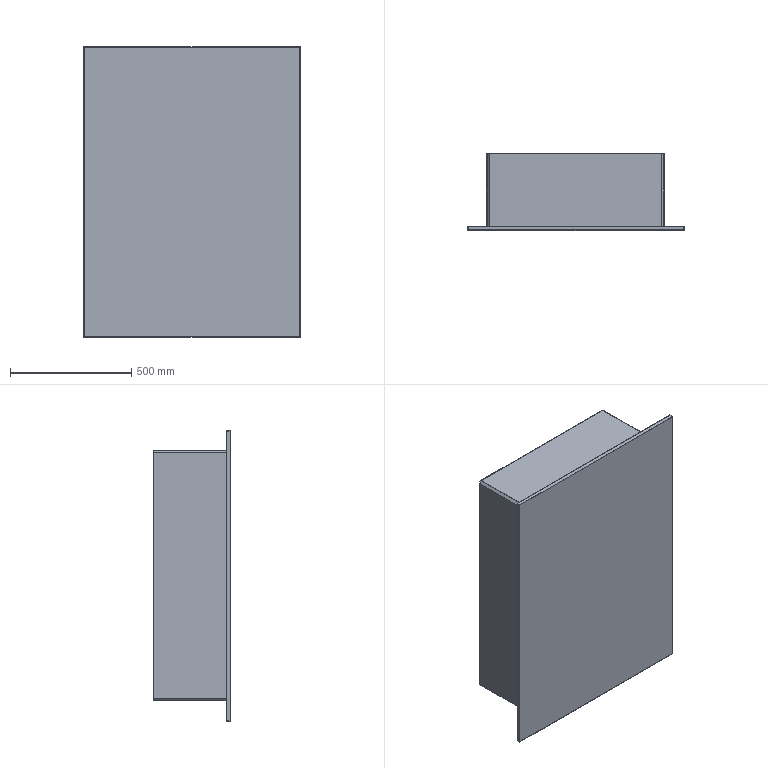Part | SolidWorks | features ICE 2, Chamfer 1, Extrusion 1, Shell 1 | 1 solid | 34 faces | box 892 x 317 x 1197 mm | volume 3890024 mm3 | plane 30 | cylinder 4 | commonest cylinder face diameters 59 x4
STEP:
#1=CARTESIAN_POINT('',(198.5,315.8,390.));
#2=VERTEX_POINT('',#1);
#3=CARTESIAN_POINT('',(198.5,315.8,449.));
#4=VERTEX_POINT('',#3);
#5=CARTESIAN_POINT('',(198.5,315.8,419.5));
#6=DIRECTION('',(0.,1.,0.));
#7=DIRECTION('',(0.,0.,1.));
#8=AXIS2_PLACEMENT_3D('',#5,#6,#7);
#9=CIRCLE('',#8,29.5);
#10=EDGE_CURVE('',#2,#4,#9,.T.);
#11=ORIENTED_EDGE('',*,*,#10,.F.);
#12=CARTESIAN_POINT('',(198.5,317.,390.));
#13=VERTEX_POINT('',#12);
#14=CARTESIAN_POINT('',(198.5,307.,390.));
#15=DIRECTION('',(0.,1.,0.));
#16=VECTOR('',#15,1000.);
#17=LINE('',#14,#16);
#18=EDGE_CURVE('',#2,#13,#17,.T.);
#19=ORIENTED_EDGE('',*,*,#18,.T.);
#20=CARTESIAN_POINT('',(198.5,317.,449.));
#21=VERTEX_POINT('',#20);
#22=CARTESIAN_POINT('',(198.5,317.,419.5));
#23=DIRECTION('',(0.,1.,0.));
#24=DIRECTION('',(0.,0.,1.));
#25=AXIS2_PLACEMENT_3D('',#22,#23,#24);
#26=CIRCLE('',#25,29.5);
#27=EDGE_CURVE('',#13,#21,#26,.T.);
#28=ORIENTED_EDGE('',*,*,#27,.T.);
#29=CARTESIAN_POINT('',(198.5,307.,449.));
#30=DIRECTION('',(0.,1.,0.));
#31=VECTOR('',#30,1000.);
#32=LINE('',#29,#31);
#33=EDGE_CURVE('',#4,#21,#32,.T.);
#34=ORIENTED_EDGE('',*,*,#33,.F.);
#35=EDGE_LOOP('',(#11,#19,#28,#34));
#36=FACE_OUTER_BOUND('',#35,.T.);
#37=CARTESIAN_POINT('',(198.5,307.,419.5));
#38=DIRECTION('',(0.,1.,0.));
#39=DIRECTION('',(0.,0.,1.));
#40=AXIS2_PLACEMENT_3D('',#37,#38,#39);
#41=CYLINDRICAL_SURFACE('',#40,29.5);
#42=ADVANCED_FACE('',(#36),#41,.F.);
#43=CARTESIAN_POINT('',(-201.5,315.8,390.));
#44=VERTEX_POINT('',#43);
#45=CARTESIAN_POINT('',(-201.5,315.8,449.));
#46=VERTEX_POINT('',#45);
#47=CARTESIAN_POINT('',(-201.5,315.8,419.5));
#48=DIRECTION('',(0.,1.,0.));
#49=DIRECTION('',(0.,0.,1.));
#50=AXIS2_PLACEMENT_3D('',#47,#48,#49);
#51=CIRCLE('',#50,29.5);
#52=EDGE_CURVE('',#44,#46,#51,.T.);
#53=ORIENTED_EDGE('',*,*,#52,.F.);
#54=CARTESIAN_POINT('',(-201.5,317.,390.));
#55=VERTEX_POINT('',#54);
#56=CARTESIAN_POINT('',(-201.5,307.,390.));
#57=DIRECTION('',(0.,1.,0.));
#58=VECTOR('',#57,1000.);
#59=LINE('',#56,#58);
#60=EDGE_CURVE('',#44,#55,#59,.T.);
#61=ORIENTED_EDGE('',*,*,#60,.T.);
#62=CARTESIAN_POINT('',(-201.5,317.,449.));
#63=VERTEX_POINT('',#62);
#64=CARTESIAN_POINT('',(-201.5,317.,419.5));
#65=DIRECTION('',(0.,1.,0.));
#66=DIRECTION('',(0.,0.,1.));
#67=AXIS2_PLACEMENT_3D('',#64,#65,#66);
#68=CIRCLE('',#67,29.5);
#69=EDGE_CURVE('',#55,#63,#68,.T.);
#70=ORIENTED_EDGE('',*,*,#69,.T.);
#71=CARTESIAN_POINT('',(-201.5,307.,449.));
#72=DIRECTION('',(0.,1.,0.));
#73=VECTOR('',#72,1000.);
#74=LINE('',#71,#73);
#75=EDGE_CURVE('',#46,#63,#74,.T.);
#76=ORIENTED_EDGE('',*,*,#75,.F.);
#77=EDGE_LOOP('',(#53,#61,#70,#76));
#78=FACE_OUTER_BOUND('',#77,.T.);
#79=CARTESIAN_POINT('',(-201.5,307.,419.5));
#80=DIRECTION('',(0.,1.,0.));
#81=DIRECTION('',(0.,0.,1.));
#82=AXIS2_PLACEMENT_3D('',#79,#80,#81);
#83=CYLINDRICAL_SURFACE('',#82,29.5);
#84=ADVANCED_FACE('',(#78),#83,.F.);
#85=CARTESIAN_POINT('',(444.8,15.8,597.3));
#86=VERTEX_POINT('',#85);
#87=CARTESIAN_POINT('',(444.8,15.8,-597.3));
#88=VERTEX_POINT('',#87);
#89=CARTESIAN_POINT('',(444.8,15.8,0.));
#90=DIRECTION('',(0.,0.,-1.));
#91=VECTOR('',#90,1000.);
#92=LINE('',#89,#91);
#93=EDGE_CURVE('',#86,#88,#92,.T.);
#94=ORIENTED_EDGE('',*,*,#93,.F.);
#95=CARTESIAN_POINT('',(-444.8,15.8,597.3));
#96=VERTEX_POINT('',#95);
#97=CARTESIAN_POINT('',(0.,15.8,597.3));
#98=DIRECTION('',(1.,0.,0.));
#99=VECTOR('',#98,1000.);
#100=LINE('',#97,#99);
#101=EDGE_CURVE('',#96,#86,#100,.T.);
#102=ORIENTED_EDGE('',*,*,#101,.F.);
#103=CARTESIAN_POINT('',(-444.8,15.8,-597.3));
#104=VERTEX_POINT('',#103);
#105=CARTESIAN_POINT('',(-444.8,15.8,0.));
#106=DIRECTION('',(0.,0.,1.));
#107=VECTOR('',#106,1000.);
#108=LINE('',#105,#107);
#109=EDGE_CURVE('',#104,#96,#108,.T.);
#110=ORIENTED_EDGE('',*,*,#109,.F.);
#111=CARTESIAN_POINT('',(0.,15.8,-597.3));
#112=DIRECTION('',(-1.,0.,0.));
#113=VECTOR('',#112,1000.);
#114=LINE('',#111,#113);
#115=EDGE_CURVE('',#88,#104,#114,.T.);
#116=ORIENTED_EDGE('',*,*,#115,.F.);
#117=EDGE_LOOP('',(#94,#102,#110,#116));
#118=FACE_OUTER_BOUND('',#117,.T.);
#119=CARTESIAN_POINT('',(362.8,15.8,509.003));
#120=VERTEX_POINT('',#119);
#121=CARTESIAN_POINT('',(362.8,15.8,-504.003));
#122=VERTEX_POINT('',#121);
#123=CARTESIAN_POINT('',(362.8,15.8,0.));
#124=DIRECTION('',(0.,0.,-1.));
#125=VECTOR('',#124,1000.);
#126=LINE('',#123,#125);
#127=EDGE_CURVE('',#120,#122,#126,.T.);
#128=ORIENTED_EDGE('',*,*,#127,.T.);
#129=CARTESIAN_POINT('',(353.503,15.8,-513.3));
#130=VERTEX_POINT('',#129);
#131=CARTESIAN_POINT('',(433.401,15.8,-433.401));
#132=DIRECTION('',(0.7071,0.,0.7071));
#133=VECTOR('',#132,1000.);
#134=LINE('',#131,#133);
#135=EDGE_CURVE('',#130,#122,#134,.T.);
#136=ORIENTED_EDGE('',*,*,#135,.F.);
#137=CARTESIAN_POINT('',(-356.503,15.8,-513.3));
#138=VERTEX_POINT('',#137);
#139=CARTESIAN_POINT('',(0.,15.8,-513.3));
#140=DIRECTION('',(-1.,0.,0.));
#141=VECTOR('',#140,1000.);
#142=LINE('',#139,#141);
#143=EDGE_CURVE('',#130,#138,#142,.T.);
#144=ORIENTED_EDGE('',*,*,#143,.T.);
#145=CARTESIAN_POINT('',(-365.8,15.8,-504.003));
#146=VERTEX_POINT('',#145);
#147=CARTESIAN_POINT('',(-434.901,15.8,-434.901));
#148=DIRECTION('',(0.7071,0.,-0.7071));
#149=VECTOR('',#148,1000.);
#150=LINE('',#147,#149);
#151=EDGE_CURVE('',#146,#138,#150,.T.);
#152=ORIENTED_EDGE('',*,*,#151,.F.);
#153=CARTESIAN_POINT('',(-365.8,15.8,509.003));
#154=VERTEX_POINT('',#153);
#155=CARTESIAN_POINT('',(-365.8,15.8,0.));
#156=DIRECTION('',(0.,0.,1.));
#157=VECTOR('',#156,1000.);
#158=LINE('',#155,#157);
#159=EDGE_CURVE('',#146,#154,#158,.T.);
#160=ORIENTED_EDGE('',*,*,#159,.T.);
#161=CARTESIAN_POINT('',(-356.503,15.8,518.3));
#162=VERTEX_POINT('',#161);
#163=CARTESIAN_POINT('',(-437.401,15.8,437.401));
#164=DIRECTION('',(-0.7071,0.,-0.7071));
#165=VECTOR('',#164,1000.);
#166=LINE('',#163,#165);
#167=EDGE_CURVE('',#162,#154,#166,.T.);
#168=ORIENTED_EDGE('',*,*,#167,.F.);
#169=CARTESIAN_POINT('',(353.503,15.8,518.3));
#170=VERTEX_POINT('',#169);
#171=CARTESIAN_POINT('',(0.,15.8,518.3));
#172=DIRECTION('',(1.,0.,0.));
#173=VECTOR('',#172,1000.);
#174=LINE('',#171,#173);
#175=EDGE_CURVE('',#162,#170,#174,.T.);
#176=ORIENTED_EDGE('',*,*,#175,.T.);
#177=CARTESIAN_POINT('',(435.901,15.8,435.901));
#178=DIRECTION('',(-0.7071,0.,0.7071));
#179=VECTOR('',#178,1000.);
#180=LINE('',#177,#179);
#181=EDGE_CURVE('',#120,#170,#180,.T.);
#182=ORIENTED_EDGE('',*,*,#181,.F.);
#183=EDGE_LOOP('',(#128,#136,#144,#152,#160,#168,#176,#182));
#184=FACE_BOUND('',#183,.T.);
#185=CARTESIAN_POINT('',(0.,15.8,0.));
#186=DIRECTION('',(0.,-1.,0.));
#187=DIRECTION('',(0.,0.,-1.));
#188=AXIS2_PLACEMENT_3D('',#185,#186,#187);
#189=PLANE('',#188);
#190=ADVANCED_FACE('',(#118,#184),#189,.T.);
#191=CARTESIAN_POINT('',(444.8,1.2,597.3));
#192=VERTEX_POINT('',#191);
#193=CARTESIAN_POINT('',(444.8,1.2,-597.3));
#194=VERTEX_POINT('',#193);
#195=CARTESIAN_POINT('',(444.8,1.2,0.));
#196=DIRECTION('',(0.,0.,-1.));
#197=VECTOR('',#196,1000.);
#198=LINE('',#195,#197);
#199=EDGE_CURVE('',#192,#194,#198,.T.);
#200=ORIENTED_EDGE('',*,*,#199,.F.);
#201=CARTESIAN_POINT('',(444.8,17.,597.3));
#202=DIRECTION('',(0.,-1.,0.));
#203=VECTOR('',#202,1000.);
#204=LINE('',#201,#203);
#205=EDGE_CURVE('',#86,#192,#204,.T.);
#206=ORIENTED_EDGE('',*,*,#205,.F.);
#207=ORIENTED_EDGE('',*,*,#93,.T.);
#208=CARTESIAN_POINT('',(444.8,17.,-597.3));
#209=DIRECTION('',(0.,-1.,0.));
#210=VECTOR('',#209,1000.);
#211=LINE('',#208,#210);
#212=EDGE_CURVE('',#88,#194,#211,.T.);
#213=ORIENTED_EDGE('',*,*,#212,.T.);
#214=EDGE_LOOP('',(#200,#206,#207,#213));
#215=FACE_OUTER_BOUND('',#214,.T.);
#216=CARTESIAN_POINT('',(444.8,17.,598.5));
#217=DIRECTION('',(-1.,0.,0.));
#218=DIRECTION('',(0.,0.,1.));
#219=AXIS2_PLACEMENT_3D('',#216,#217,#218);
#220=PLANE('',#219);
#221=ADVANCED_FACE('',(#215),#220,.T.);
#222=CARTESIAN_POINT('',(-444.8,1.2,-597.3));
#223=VERTEX_POINT('',#222);
#224=CARTESIAN_POINT('',(0.,1.2,-597.3));
#225=DIRECTION('',(-1.,0.,0.));
#226=VECTOR('',#225,1000.);
#227=LINE('',#224,#226);
#228=EDGE_CURVE('',#194,#223,#227,.T.);
#229=ORIENTED_EDGE('',*,*,#228,.F.);
#230=ORIENTED_EDGE('',*,*,#212,.F.);
#231=ORIENTED_EDGE('',*,*,#115,.T.);
#232=CARTESIAN_POINT('',(-444.8,17.,-597.3));
#233=DIRECTION('',(0.,-1.,0.));
#234=VECTOR('',#233,1000.);
#235=LINE('',#232,#234);
#236=EDGE_CURVE('',#104,#223,#235,.T.);
#237=ORIENTED_EDGE('',*,*,#236,.T.);
#238=EDGE_LOOP('',(#229,#230,#231,#237));
#239=FACE_OUTER_BOUND('',#238,.T.);
#240=CARTESIAN_POINT('',(-446.,17.,-597.3));
#241=DIRECTION('',(0.,0.,1.));
#242=DIRECTION('',(1.,0.,0.));
#243=AXIS2_PLACEMENT_3D('',#240,#241,#242);
#244=PLANE('',#243);
#245=ADVANCED_FACE('',(#239),#244,.T.);
#246=CARTESIAN_POINT('',(-444.8,1.2,597.3));
#247=VERTEX_POINT('',#246);
#248=CARTESIAN_POINT('',(-444.8,1.2,0.));
#249=DIRECTION('',(0.,0.,1.));
#250=VECTOR('',#249,1000.);
#251=LINE('',#248,#250);
#252=EDGE_CURVE('',#223,#247,#251,.T.);
#253=ORIENTED_EDGE('',*,*,#252,.F.);
#254=ORIENTED_EDGE('',*,*,#236,.F.);
#255=ORIENTED_EDGE('',*,*,#109,.T.);
#256=CARTESIAN_POINT('',(-444.8,17.,597.3));
#257=DIRECTION('',(0.,-1.,0.));
#258=VECTOR('',#257,1000.);
#259=LINE('',#256,#258);
#260=EDGE_CURVE('',#96,#247,#259,.T.);
#261=ORIENTED_EDGE('',*,*,#260,.T.);
#262=EDGE_LOOP('',(#253,#254,#255,#261));
#263=FACE_OUTER_BOUND('',#262,.T.);
#264=CARTESIAN_POINT('',(-444.8,17.,598.5));
#265=DIRECTION('',(1.,0.,0.));
#266=DIRECTION('',(0.,0.,-1.));
#267=AXIS2_PLACEMENT_3D('',#264,#265,#266);
#268=PLANE('',#267);
#269=ADVANCED_FACE('',(#263),#268,.T.);
#270=CARTESIAN_POINT('',(0.,1.2,597.3));
#271=DIRECTION('',(1.,0.,0.));
#272=VECTOR('',#271,1000.);
#273=LINE('',#270,#272);
#274=EDGE_CURVE('',#247,#192,#273,.T.);
#275=ORIENTED_EDGE('',*,*,#274,.F.);
#276=ORIENTED_EDGE('',*,*,#260,.F.);
#277=ORIENTED_EDGE('',*,*,#101,.T.);
#278=ORIENTED_EDGE('',*,*,#205,.T.);
#279=EDGE_LOOP('',(#275,#276,#277,#278));
#280=FACE_OUTER_BOUND('',#279,.T.);
#281=CARTESIAN_POINT('',(-446.,17.,597.3));
#282=DIRECTION('',(0.,0.,-1.));
#283=DIRECTION('',(-1.,0.,0.));
#284=AXIS2_PLACEMENT_3D('',#281,#282,#283);
#285=PLANE('',#284);
#286=ADVANCED_FACE('',(#280),#285,.T.);
#287=ORIENTED_EDGE('',*,*,#199,.T.);
#288=ORIENTED_EDGE('',*,*,#228,.T.);
#289=ORIENTED_EDGE('',*,*,#252,.T.);
#290=ORIENTED_EDGE('',*,*,#274,.T.);
#291=EDGE_LOOP('',(#287,#288,#289,#290));
#292=FACE_OUTER_BOUND('',#291,.T.);
#293=CARTESIAN_POINT('',(0.,1.2,0.));
#294=DIRECTION('',(0.,-1.,0.));
#295=DIRECTION('',(0.,0.,-1.));
#296=AXIS2_PLACEMENT_3D('',#293,#294,#295);
#297=PLANE('',#296);
#298=ADVANCED_FACE('',(#292),#297,.F.);
#299=ORIENTED_EDGE('',*,*,#127,.F.);
#300=CARTESIAN_POINT('',(362.8,315.8,509.003));
#301=VERTEX_POINT('',#300);
#302=CARTESIAN_POINT('',(362.8,317.,509.003));
#303=DIRECTION('',(0.,-1.,0.));
#304=VECTOR('',#303,1000.);
#305=LINE('',#302,#304);
#306=EDGE_CURVE('',#301,#120,#305,.T.);
#307=ORIENTED_EDGE('',*,*,#306,.F.);
#308=CARTESIAN_POINT('',(362.8,315.8,-504.003));
#309=VERTEX_POINT('',#308);
#310=CARTESIAN_POINT('',(362.8,315.8,519.5));
#311=DIRECTION('',(0.,0.,-1.));
#312=VECTOR('',#311,1000.);
#313=LINE('',#310,#312);
#314=EDGE_CURVE('',#301,#309,#313,.T.);
#315=ORIENTED_EDGE('',*,*,#314,.T.);
#316=CARTESIAN_POINT('',(362.8,317.,-504.003));
#317=DIRECTION('',(0.,1.,0.));
#318=VECTOR('',#317,1000.);
#319=LINE('',#316,#318);
#320=EDGE_CURVE('',#122,#309,#319,.T.);
#321=ORIENTED_EDGE('',*,*,#320,.F.);
#322=EDGE_LOOP('',(#299,#307,#315,#321));
#323=FACE_OUTER_BOUND('',#322,.T.);
#324=CARTESIAN_POINT('',(362.8,317.,519.5));
#325=DIRECTION('',(-1.,0.,0.));
#326=DIRECTION('',(0.,0.,1.));
#327=AXIS2_PLACEMENT_3D('',#324,#325,#326);
#328=PLANE('',#327);
#329=ADVANCED_FACE('',(#323),#328,.T.);
#330=CARTESIAN_POINT('',(353.503,315.8,-513.3));
#331=VERTEX_POINT('',#330);
#332=CARTESIAN_POINT('',(-356.503,315.8,-513.3));
#333=VERTEX_POINT('',#332);
#334=CARTESIAN_POINT('',(364.,315.8,-513.3));
#335=DIRECTION('',(-1.,0.,0.));
#336=VECTOR('',#335,1000.);
#337=LINE('',#334,#336);
#338=EDGE_CURVE('',#331,#333,#337,.T.);
#339=ORIENTED_EDGE('',*,*,#338,.T.);
#340=CARTESIAN_POINT('',(-356.503,317.,-513.3));
#341=DIRECTION('',(0.,1.,0.));
#342=VECTOR('',#341,1000.);
#343=LINE('',#340,#342);
#344=EDGE_CURVE('',#138,#333,#343,.T.);
#345=ORIENTED_EDGE('',*,*,#344,.F.);
#346=ORIENTED_EDGE('',*,*,#143,.F.);
#347=CARTESIAN_POINT('',(353.503,317.,-513.3));
#348=DIRECTION('',(0.,-1.,0.));
#349=VECTOR('',#348,1000.);
#350=LINE('',#347,#349);
#351=EDGE_CURVE('',#331,#130,#350,.T.);
#352=ORIENTED_EDGE('',*,*,#351,.F.);
#353=EDGE_LOOP('',(#339,#345,#346,#352));
#354=FACE_OUTER_BOUND('',#353,.T.);
#355=CARTESIAN_POINT('',(364.,317.,-513.3));
#356=DIRECTION('',(0.,0.,1.));
#357=DIRECTION('',(1.,0.,0.));
#358=AXIS2_PLACEMENT_3D('',#355,#356,#357);
#359=PLANE('',#358);
#360=ADVANCED_FACE('',(#354),#359,.T.);
#361=CARTESIAN_POINT('',(-365.8,315.8,-504.003));
#362=VERTEX_POINT('',#361);
#363=CARTESIAN_POINT('',(-365.8,315.8,509.003));
#364=VERTEX_POINT('',#363);
#365=CARTESIAN_POINT('',(-365.8,315.8,519.5));
#366=DIRECTION('',(0.,0.,1.));
#367=VECTOR('',#366,1000.);
#368=LINE('',#365,#367);
#369=EDGE_CURVE('',#362,#364,#368,.T.);
#370=ORIENTED_EDGE('',*,*,#369,.T.);
#371=CARTESIAN_POINT('',(-365.8,317.,509.003));
#372=DIRECTION('',(0.,1.,0.));
#373=VECTOR('',#372,1000.);
#374=LINE('',#371,#373);
#375=EDGE_CURVE('',#154,#364,#374,.T.);
#376=ORIENTED_EDGE('',*,*,#375,.F.);
#377=ORIENTED_EDGE('',*,*,#159,.F.);
#378=CARTESIAN_POINT('',(-365.8,317.,-504.003));
#379=DIRECTION('',(0.,-1.,0.));
#380=VECTOR('',#379,1000.);
#381=LINE('',#378,#380);
#382=EDGE_CURVE('',#362,#146,#381,.T.);
#383=ORIENTED_EDGE('',*,*,#382,.F.);
#384=EDGE_LOOP('',(#370,#376,#377,#383));
#385=FACE_OUTER_BOUND('',#384,.T.);
#386=CARTESIAN_POINT('',(-365.8,317.,519.5));
#387=DIRECTION('',(1.,0.,0.));
#388=DIRECTION('',(0.,0.,-1.));
#389=AXIS2_PLACEMENT_3D('',#386,#387,#388);
#390=PLANE('',#389);
#391=ADVANCED_FACE('',(#385),#390,.T.);
#392=ORIENTED_EDGE('',*,*,#175,.F.);
#393=CARTESIAN_POINT('',(-356.503,315.8,518.3));
#394=VERTEX_POINT('',#393);
#395=CARTESIAN_POINT('',(-356.503,317.,518.3));
#396=DIRECTION('',(0.,-1.,0.));
#397=VECTOR('',#396,1000.);
#398=LINE('',#395,#397);
#399=EDGE_CURVE('',#394,#162,#398,.T.);
#400=ORIENTED_EDGE('',*,*,#399,.F.);
#401=CARTESIAN_POINT('',(353.503,315.8,518.3));
#402=VERTEX_POINT('',#401);
#403=CARTESIAN_POINT('',(364.,315.8,518.3));
#404=DIRECTION('',(1.,0.,0.));
#405=VECTOR('',#404,1000.);
#406=LINE('',#403,#405);
#407=EDGE_CURVE('',#394,#402,#406,.T.);
#408=ORIENTED_EDGE('',*,*,#407,.T.);
#409=CARTESIAN_POINT('',(353.503,317.,518.3));
#410=DIRECTION('',(0.,1.,0.));
#411=VECTOR('',#410,1000.);
#412=LINE('',#409,#411);
#413=EDGE_CURVE('',#170,#402,#412,.T.);
#414=ORIENTED_EDGE('',*,*,#413,.F.);
#415=EDGE_LOOP('',(#392,#400,#408,#414));
#416=FACE_OUTER_BOUND('',#415,.T.);
#417=CARTESIAN_POINT('',(364.,317.,518.3));
#418=DIRECTION('',(0.,0.,-1.));
#419=DIRECTION('',(-1.,0.,0.));
#420=AXIS2_PLACEMENT_3D('',#417,#418,#419);
#421=PLANE('',#420);
#422=ADVANCED_FACE('',(#416),#421,.T.);
#423=CARTESIAN_POINT('',(198.5,315.8,419.5));
#424=DIRECTION('',(0.,1.,0.));
#425=DIRECTION('',(0.,0.,1.));
#426=AXIS2_PLACEMENT_3D('',#423,#424,#425);
#427=CIRCLE('',#426,29.5);
#428=EDGE_CURVE('',#4,#2,#427,.T.);
#429=ORIENTED_EDGE('',*,*,#428,.T.);
#430=ORIENTED_EDGE('',*,*,#10,.T.);
#431=EDGE_LOOP('',(#429,#430));
#432=FACE_BOUND('',#431,.T.);
#433=CARTESIAN_POINT('',(-201.5,315.8,419.5));
#434=DIRECTION('',(0.,1.,0.));
#435=DIRECTION('',(0.,0.,1.));
#436=AXIS2_PLACEMENT_3D('',#433,#434,#435);
#437=CIRCLE('',#436,29.5);
#438=EDGE_CURVE('',#46,#44,#437,.T.);
#439=ORIENTED_EDGE('',*,*,#438,.T.);
#440=ORIENTED_EDGE('',*,*,#52,.T.);
#441=EDGE_LOOP('',(#439,#440));
#442=FACE_BOUND('',#441,.T.);
#443=ORIENTED_EDGE('',*,*,#314,.F.);
#444=CARTESIAN_POINT('',(435.901,315.8,435.901));
#445=DIRECTION('',(0.7071,0.,-0.7071));
#446=VECTOR('',#445,1000.);
#447=LINE('',#444,#446);
#448=EDGE_CURVE('',#402,#301,#447,.T.);
#449=ORIENTED_EDGE('',*,*,#448,.F.);
#450=ORIENTED_EDGE('',*,*,#407,.F.);
#451=CARTESIAN_POINT('',(-437.401,315.8,437.401));
#452=DIRECTION('',(0.7071,0.,0.7071));
#453=VECTOR('',#452,1000.);
#454=LINE('',#451,#453);
#455=EDGE_CURVE('',#364,#394,#454,.T.);
#456=ORIENTED_EDGE('',*,*,#455,.F.);
#457=ORIENTED_EDGE('',*,*,#369,.F.);
#458=CARTESIAN_POINT('',(-434.901,315.8,-434.901));
#459=DIRECTION('',(-0.7071,0.,0.7071));
#460=VECTOR('',#459,1000.);
#461=LINE('',#458,#460);
#462=EDGE_CURVE('',#333,#362,#461,.T.);
#463=ORIENTED_EDGE('',*,*,#462,.F.);
#464=ORIENTED_EDGE('',*,*,#338,.F.);
#465=CARTESIAN_POINT('',(433.401,315.8,-433.401));
#466=DIRECTION('',(-0.7071,0.,-0.7071));
#467=VECTOR('',#466,1000.);
#468=LINE('',#465,#467);
#469=EDGE_CURVE('',#309,#331,#468,.T.);
#470=ORIENTED_EDGE('',*,*,#469,.F.);
#471=EDGE_LOOP('',(#443,#449,#450,#456,#457,#463,#464,#470));
#472=FACE_OUTER_BOUND('',#471,.T.);
#473=CARTESIAN_POINT('',(0.,315.8,0.));
#474=DIRECTION('',(0.,1.,0.));
#475=DIRECTION('',(0.,0.,1.));
#476=AXIS2_PLACEMENT_3D('',#473,#474,#475);
#477=PLANE('',#476);
#478=ADVANCED_FACE('',(#432,#442,#472),#477,.F.);
#479=ORIENTED_EDGE('',*,*,#469,.T.);
#480=ORIENTED_EDGE('',*,*,#351,.T.);
#481=ORIENTED_EDGE('',*,*,#135,.T.);
#482=ORIENTED_EDGE('',*,*,#320,.T.);
#483=EDGE_LOOP('',(#479,#480,#481,#482));
#484=FACE_OUTER_BOUND('',#483,.T.);
#485=CARTESIAN_POINT('',(353.151,317.,-513.651));
#486=DIRECTION('',(-0.7071,0.,0.7071));
#487=DIRECTION('',(0.,-1.,0.));
#488=AXIS2_PLACEMENT_3D('',#485,#486,#487);
#489=PLANE('',#488);
#490=ADVANCED_FACE('',(#484),#489,.T.);
#491=ORIENTED_EDGE('',*,*,#462,.T.);
#492=ORIENTED_EDGE('',*,*,#382,.T.);
#493=ORIENTED_EDGE('',*,*,#151,.T.);
#494=ORIENTED_EDGE('',*,*,#344,.T.);
#495=EDGE_LOOP('',(#491,#492,#493,#494));
#496=FACE_OUTER_BOUND('',#495,.T.);
#497=CARTESIAN_POINT('',(-366.151,317.,-503.651));
#498=DIRECTION('',(0.7071,0.,0.7071));
#499=DIRECTION('',(0.,-1.,0.));
#500=AXIS2_PLACEMENT_3D('',#497,#498,#499);
#501=PLANE('',#500);
#502=ADVANCED_FACE('',(#496),#501,.T.);
#503=ORIENTED_EDGE('',*,*,#448,.T.);
#504=ORIENTED_EDGE('',*,*,#306,.T.);
#505=ORIENTED_EDGE('',*,*,#181,.T.);
#506=ORIENTED_EDGE('',*,*,#413,.T.);
#507=EDGE_LOOP('',(#503,#504,#505,#506));
#508=FACE_OUTER_BOUND('',#507,.T.);
#509=CARTESIAN_POINT('',(363.151,317.,508.651));
#510=DIRECTION('',(-0.7071,0.,-0.7071));
#511=DIRECTION('',(0.,-1.,0.));
#512=AXIS2_PLACEMENT_3D('',#509,#510,#511);
#513=PLANE('',#512);
#514=ADVANCED_FACE('',(#508),#513,.T.);
#515=ORIENTED_EDGE('',*,*,#455,.T.);
#516=ORIENTED_EDGE('',*,*,#399,.T.);
#517=ORIENTED_EDGE('',*,*,#167,.T.);
#518=ORIENTED_EDGE('',*,*,#375,.T.);
#519=EDGE_LOOP('',(#515,#516,#517,#518));
#520=FACE_OUTER_BOUND('',#519,.T.);
#521=CARTESIAN_POINT('',(-356.151,317.,518.651));
#522=DIRECTION('',(0.7071,0.,-0.7071));
#523=DIRECTION('',(0.,-1.,0.));
#524=AXIS2_PLACEMENT_3D('',#521,#522,#523);
#525=PLANE('',#524);
#526=ADVANCED_FACE('',(#520),#525,.T.);
#527=ORIENTED_EDGE('',*,*,#60,.F.);
#528=ORIENTED_EDGE('',*,*,#438,.F.);
#529=ORIENTED_EDGE('',*,*,#75,.T.);
#530=CARTESIAN_POINT('',(-201.5,317.,419.5));
#531=DIRECTION('',(0.,1.,0.));
#532=DIRECTION('',(0.,0.,1.));
#533=AXIS2_PLACEMENT_3D('',#530,#531,#532);
#534=CIRCLE('',#533,29.5);
#535=EDGE_CURVE('',#63,#55,#534,.T.);
#536=ORIENTED_EDGE('',*,*,#535,.T.);
#537=EDGE_LOOP('',(#527,#528,#529,#536));
#538=FACE_OUTER_BOUND('',#537,.T.);
#539=CARTESIAN_POINT('',(-201.5,307.,419.5));
#540=DIRECTION('',(0.,1.,0.));
#541=DIRECTION('',(0.,0.,1.));
#542=AXIS2_PLACEMENT_3D('',#539,#540,#541);
#543=CYLINDRICAL_SURFACE('',#542,29.5);
#544=ADVANCED_FACE('',(#538),#543,.F.);
#545=ORIENTED_EDGE('',*,*,#18,.F.);
#546=ORIENTED_EDGE('',*,*,#428,.F.);
#547=ORIENTED_EDGE('',*,*,#33,.T.);
#548=CARTESIAN_POINT('',(198.5,317.,419.5));
#549=DIRECTION('',(0.,1.,0.));
#550=DIRECTION('',(0.,0.,1.));
#551=AXIS2_PLACEMENT_3D('',#548,#549,#550);
#552=CIRCLE('',#551,29.5);
#553=EDGE_CURVE('',#21,#13,#552,.T.);
#554=ORIENTED_EDGE('',*,*,#553,.T.);
#555=EDGE_LOOP('',(#545,#546,#547,#554));
#556=FACE_OUTER_BOUND('',#555,.T.);
#557=CARTESIAN_POINT('',(198.5,307.,419.5));
#558=DIRECTION('',(0.,1.,0.));
#559=DIRECTION('',(0.,0.,1.));
#560=AXIS2_PLACEMENT_3D('',#557,#558,#559);
#561=CYLINDRICAL_SURFACE('',#560,29.5);
#562=ADVANCED_FACE('',(#556),#561,.F.);
#563=CARTESIAN_POINT('',(446.,17.,598.5));
#564=VERTEX_POINT('',#563);
#565=CARTESIAN_POINT('',(446.,17.,-598.5));
#566=VERTEX_POINT('',#565);
#567=CARTESIAN_POINT('',(446.,17.,598.5));
#568=DIRECTION('',(0.,0.,-1.));
#569=VECTOR('',#568,1000.);
#570=LINE('',#567,#569);
#571=EDGE_CURVE('',#564,#566,#570,.T.);
#572=ORIENTED_EDGE('',*,*,#571,.T.);
#573=CARTESIAN_POINT('',(-446.,17.,-598.5));
#574=VERTEX_POINT('',#573);
#575=CARTESIAN_POINT('',(-446.,17.,-598.5));
#576=DIRECTION('',(-1.,0.,0.));
#577=VECTOR('',#576,1000.);
#578=LINE('',#575,#577);
#579=EDGE_CURVE('',#566,#574,#578,.T.);
#580=ORIENTED_EDGE('',*,*,#579,.T.);
#581=CARTESIAN_POINT('',(-446.,17.,598.5));
#582=VERTEX_POINT('',#581);
#583=CARTESIAN_POINT('',(-446.,17.,598.5));
#584=DIRECTION('',(0.,0.,1.));
#585=VECTOR('',#584,1000.);
#586=LINE('',#583,#585);
#587=EDGE_CURVE('',#574,#582,#586,.T.);
#588=ORIENTED_EDGE('',*,*,#587,.T.);
#589=CARTESIAN_POINT('',(-446.,17.,598.5));
#590=DIRECTION('',(1.,0.,0.));
#591=VECTOR('',#590,1000.);
#592=LINE('',#589,#591);
#593=EDGE_CURVE('',#582,#564,#592,.T.);
#594=ORIENTED_EDGE('',*,*,#593,.T.);
#595=EDGE_LOOP('',(#572,#580,#588,#594));
#596=FACE_OUTER_BOUND('',#595,.T.);
#597=CARTESIAN_POINT('',(364.,17.,509.5));
#598=VERTEX_POINT('',#597);
#599=CARTESIAN_POINT('',(364.,17.,-504.5));
#600=VERTEX_POINT('',#599);
#601=CARTESIAN_POINT('',(364.,17.,519.5));
#602=DIRECTION('',(0.,0.,-1.));
#603=VECTOR('',#602,1000.);
#604=LINE('',#601,#603);
#605=EDGE_CURVE('',#598,#600,#604,.T.);
#606=ORIENTED_EDGE('',*,*,#605,.F.);
#607=CARTESIAN_POINT('',(354.,17.,519.5));
#608=VERTEX_POINT('',#607);
#609=CARTESIAN_POINT('',(436.75,17.,436.75));
#610=DIRECTION('',(-0.7071,0.,0.7071));
#611=VECTOR('',#610,1000.);
#612=LINE('',#609,#611);
#613=EDGE_CURVE('',#598,#608,#612,.T.);
#614=ORIENTED_EDGE('',*,*,#613,.T.);
#615=CARTESIAN_POINT('',(-357.,17.,519.5));
#616=VERTEX_POINT('',#615);
#617=CARTESIAN_POINT('',(364.,17.,519.5));
#618=DIRECTION('',(1.,0.,0.));
#619=VECTOR('',#618,1000.);
#620=LINE('',#617,#619);
#621=EDGE_CURVE('',#616,#608,#620,.T.);
#622=ORIENTED_EDGE('',*,*,#621,.F.);
#623=CARTESIAN_POINT('',(-367.,17.,509.5));
#624=VERTEX_POINT('',#623);
#625=CARTESIAN_POINT('',(-438.25,17.,438.25));
#626=DIRECTION('',(-0.7071,0.,-0.7071));
#627=VECTOR('',#626,1000.);
#628=LINE('',#625,#627);
#629=EDGE_CURVE('',#616,#624,#628,.T.);
#630=ORIENTED_EDGE('',*,*,#629,.T.);
#631=CARTESIAN_POINT('',(-367.,17.,-504.5));
#632=VERTEX_POINT('',#631);
#633=CARTESIAN_POINT('',(-367.,17.,519.5));
#634=DIRECTION('',(0.,0.,1.));
#635=VECTOR('',#634,1000.);
#636=LINE('',#633,#635);
#637=EDGE_CURVE('',#632,#624,#636,.T.);
#638=ORIENTED_EDGE('',*,*,#637,.F.);
#639=CARTESIAN_POINT('',(-357.,17.,-514.5));
#640=VERTEX_POINT('',#639);
#641=CARTESIAN_POINT('',(-435.75,17.,-435.75));
#642=DIRECTION('',(0.7071,0.,-0.7071));
#643=VECTOR('',#642,1000.);
#644=LINE('',#641,#643);
#645=EDGE_CURVE('',#632,#640,#644,.T.);
#646=ORIENTED_EDGE('',*,*,#645,.T.);
#647=CARTESIAN_POINT('',(354.,17.,-514.5));
#648=VERTEX_POINT('',#647);
#649=CARTESIAN_POINT('',(364.,17.,-514.5));
#650=DIRECTION('',(-1.,0.,0.));
#651=VECTOR('',#650,1000.);
#652=LINE('',#649,#651);
#653=EDGE_CURVE('',#648,#640,#652,.T.);
#654=ORIENTED_EDGE('',*,*,#653,.F.);
#655=CARTESIAN_POINT('',(434.25,17.,-434.25));
#656=DIRECTION('',(0.7071,0.,0.7071));
#657=VECTOR('',#656,1000.);
#658=LINE('',#655,#657);
#659=EDGE_CURVE('',#648,#600,#658,.T.);
#660=ORIENTED_EDGE('',*,*,#659,.T.);
#661=EDGE_LOOP('',(#606,#614,#622,#630,#638,#646,#654,#660));
#662=FACE_BOUND('',#661,.T.);
#663=CARTESIAN_POINT('',(0.,17.,0.));
#664=DIRECTION('',(0.,-1.,0.));
#665=DIRECTION('',(0.,0.,-1.));
#666=AXIS2_PLACEMENT_3D('',#663,#664,#665);
#667=PLANE('',#666);
#668=ADVANCED_FACE('',(#596,#662),#667,.F.);
#669=CARTESIAN_POINT('',(446.,0.,598.5));
#670=VERTEX_POINT('',#669);
#671=CARTESIAN_POINT('',(446.,0.,-598.5));
#672=VERTEX_POINT('',#671);
#673=CARTESIAN_POINT('',(446.,0.,598.5));
#674=DIRECTION('',(0.,0.,-1.));
#675=VECTOR('',#674,1000.);
#676=LINE('',#673,#675);
#677=EDGE_CURVE('',#670,#672,#676,.T.);
#678=ORIENTED_EDGE('',*,*,#677,.T.);
#679=CARTESIAN_POINT('',(446.,17.,-598.5));
#680=DIRECTION('',(0.,-1.,0.));
#681=VECTOR('',#680,1000.);
#682=LINE('',#679,#681);
#683=EDGE_CURVE('',#566,#672,#682,.T.);
#684=ORIENTED_EDGE('',*,*,#683,.F.);
#685=ORIENTED_EDGE('',*,*,#571,.F.);
#686=CARTESIAN_POINT('',(446.,17.,598.5));
#687=DIRECTION('',(0.,-1.,0.));
#688=VECTOR('',#687,1000.);
#689=LINE('',#686,#688);
#690=EDGE_CURVE('',#564,#670,#689,.T.);
#691=ORIENTED_EDGE('',*,*,#690,.T.);
#692=EDGE_LOOP('',(#678,#684,#685,#691));
#693=FACE_OUTER_BOUND('',#692,.T.);
#694=CARTESIAN_POINT('',(446.,17.,598.5));
#695=DIRECTION('',(-1.,0.,0.));
#696=DIRECTION('',(0.,0.,1.));
#697=AXIS2_PLACEMENT_3D('',#694,#695,#696);
#698=PLANE('',#697);
#699=ADVANCED_FACE('',(#693),#698,.F.);
#700=CARTESIAN_POINT('',(-446.,0.,-598.5));
#701=VERTEX_POINT('',#700);
#702=CARTESIAN_POINT('',(-446.,0.,-598.5));
#703=DIRECTION('',(-1.,0.,0.));
#704=VECTOR('',#703,1000.);
#705=LINE('',#702,#704);
#706=EDGE_CURVE('',#672,#701,#705,.T.);
#707=ORIENTED_EDGE('',*,*,#706,.T.);
#708=CARTESIAN_POINT('',(-446.,17.,-598.5));
#709=DIRECTION('',(0.,-1.,0.));
#710=VECTOR('',#709,1000.);
#711=LINE('',#708,#710);
#712=EDGE_CURVE('',#574,#701,#711,.T.);
#713=ORIENTED_EDGE('',*,*,#712,.F.);
#714=ORIENTED_EDGE('',*,*,#579,.F.);
#715=ORIENTED_EDGE('',*,*,#683,.T.);
#716=EDGE_LOOP('',(#707,#713,#714,#715));
#717=FACE_OUTER_BOUND('',#716,.T.);
#718=CARTESIAN_POINT('',(-446.,17.,-598.5));
#719=DIRECTION('',(0.,0.,1.));
#720=DIRECTION('',(1.,0.,0.));
#721=AXIS2_PLACEMENT_3D('',#718,#719,#720);
#722=PLANE('',#721);
#723=ADVANCED_FACE('',(#717),#722,.F.);
#724=CARTESIAN_POINT('',(-446.,0.,598.5));
#725=VERTEX_POINT('',#724);
#726=CARTESIAN_POINT('',(-446.,0.,598.5));
#727=DIRECTION('',(0.,0.,1.));
#728=VECTOR('',#727,1000.);
#729=LINE('',#726,#728);
#730=EDGE_CURVE('',#701,#725,#729,.T.);
#731=ORIENTED_EDGE('',*,*,#730,.T.);
#732=CARTESIAN_POINT('',(-446.,17.,598.5));
#733=DIRECTION('',(0.,-1.,0.));
#734=VECTOR('',#733,1000.);
#735=LINE('',#732,#734);
#736=EDGE_CURVE('',#582,#725,#735,.T.);
#737=ORIENTED_EDGE('',*,*,#736,.F.);
#738=ORIENTED_EDGE('',*,*,#587,.F.);
#739=ORIENTED_EDGE('',*,*,#712,.T.);
#740=EDGE_LOOP('',(#731,#737,#738,#739));
#741=FACE_OUTER_BOUND('',#740,.T.);
#742=CARTESIAN_POINT('',(-446.,17.,598.5));
#743=DIRECTION('',(1.,0.,0.));
#744=DIRECTION('',(0.,0.,-1.));
#745=AXIS2_PLACEMENT_3D('',#742,#743,#744);
#746=PLANE('',#745);
#747=ADVANCED_FACE('',(#741),#746,.F.);
#748=CARTESIAN_POINT('',(-446.,0.,598.5));
#749=DIRECTION('',(1.,0.,0.));
#750=VECTOR('',#749,1000.);
#751=LINE('',#748,#750);
#752=EDGE_CURVE('',#725,#670,#751,.T.);
#753=ORIENTED_EDGE('',*,*,#752,.T.);
#754=ORIENTED_EDGE('',*,*,#690,.F.);
#755=ORIENTED_EDGE('',*,*,#593,.F.);
#756=ORIENTED_EDGE('',*,*,#736,.T.);
#757=EDGE_LOOP('',(#753,#754,#755,#756));
#758=FACE_OUTER_BOUND('',#757,.T.);
#759=CARTESIAN_POINT('',(-446.,17.,598.5));
#760=DIRECTION('',(0.,0.,-1.));
#761=DIRECTION('',(-1.,0.,0.));
#762=AXIS2_PLACEMENT_3D('',#759,#760,#761);
#763=PLANE('',#762);
#764=ADVANCED_FACE('',(#758),#763,.F.);
#765=ORIENTED_EDGE('',*,*,#677,.F.);
#766=ORIENTED_EDGE('',*,*,#752,.F.);
#767=ORIENTED_EDGE('',*,*,#730,.F.);
#768=ORIENTED_EDGE('',*,*,#706,.F.);
#769=EDGE_LOOP('',(#765,#766,#767,#768));
#770=FACE_OUTER_BOUND('',#769,.T.);
#771=CARTESIAN_POINT('',(0.,0.,0.));
#772=DIRECTION('',(0.,-1.,0.));
#773=DIRECTION('',(0.,0.,-1.));
#774=AXIS2_PLACEMENT_3D('',#771,#772,#773);
#775=PLANE('',#774);
#776=ADVANCED_FACE('',(#770),#775,.T.);
#777=ORIENTED_EDGE('',*,*,#605,.T.);
#778=CARTESIAN_POINT('',(364.,317.,-504.5));
#779=VERTEX_POINT('',#778);
#780=CARTESIAN_POINT('',(364.,317.,-504.5));
#781=DIRECTION('',(0.,1.,0.));
#782=VECTOR('',#781,1000.);
#783=LINE('',#780,#782);
#784=EDGE_CURVE('',#600,#779,#783,.T.);
#785=ORIENTED_EDGE('',*,*,#784,.T.);
#786=CARTESIAN_POINT('',(364.,317.,509.5));
#787=VERTEX_POINT('',#786);
#788=CARTESIAN_POINT('',(364.,317.,519.5));
#789=DIRECTION('',(0.,0.,-1.));
#790=VECTOR('',#789,1000.);
#791=LINE('',#788,#790);
#792=EDGE_CURVE('',#787,#779,#791,.T.);
#793=ORIENTED_EDGE('',*,*,#792,.F.);
#794=CARTESIAN_POINT('',(364.,317.,509.5));
#795=DIRECTION('',(0.,-1.,0.));
#796=VECTOR('',#795,1000.);
#797=LINE('',#794,#796);
#798=EDGE_CURVE('',#787,#598,#797,.T.);
#799=ORIENTED_EDGE('',*,*,#798,.T.);
#800=EDGE_LOOP('',(#777,#785,#793,#799));
#801=FACE_OUTER_BOUND('',#800,.T.);
#802=CARTESIAN_POINT('',(364.,317.,519.5));
#803=DIRECTION('',(-1.,0.,0.));
#804=DIRECTION('',(0.,0.,1.));
#805=AXIS2_PLACEMENT_3D('',#802,#803,#804);
#806=PLANE('',#805);
#807=ADVANCED_FACE('',(#801),#806,.F.);
#808=CARTESIAN_POINT('',(354.,317.,-514.5));
#809=VERTEX_POINT('',#808);
#810=CARTESIAN_POINT('',(-357.,317.,-514.5));
#811=VERTEX_POINT('',#810);
#812=CARTESIAN_POINT('',(364.,317.,-514.5));
#813=DIRECTION('',(-1.,0.,0.));
#814=VECTOR('',#813,1000.);
#815=LINE('',#812,#814);
#816=EDGE_CURVE('',#809,#811,#815,.T.);
#817=ORIENTED_EDGE('',*,*,#816,.F.);
#818=CARTESIAN_POINT('',(354.,317.,-514.5));
#819=DIRECTION('',(0.,-1.,0.));
#820=VECTOR('',#819,1000.);
#821=LINE('',#818,#820);
#822=EDGE_CURVE('',#809,#648,#821,.T.);
#823=ORIENTED_EDGE('',*,*,#822,.T.);
#824=ORIENTED_EDGE('',*,*,#653,.T.);
#825=CARTESIAN_POINT('',(-357.,317.,-514.5));
#826=DIRECTION('',(0.,1.,0.));
#827=VECTOR('',#826,1000.);
#828=LINE('',#825,#827);
#829=EDGE_CURVE('',#640,#811,#828,.T.);
#830=ORIENTED_EDGE('',*,*,#829,.T.);
#831=EDGE_LOOP('',(#817,#823,#824,#830));
#832=FACE_OUTER_BOUND('',#831,.T.);
#833=CARTESIAN_POINT('',(364.,317.,-514.5));
#834=DIRECTION('',(0.,0.,1.));
#835=DIRECTION('',(1.,0.,0.));
#836=AXIS2_PLACEMENT_3D('',#833,#834,#835);
#837=PLANE('',#836);
#838=ADVANCED_FACE('',(#832),#837,.F.);
#839=CARTESIAN_POINT('',(-367.,317.,-504.5));
#840=VERTEX_POINT('',#839);
#841=CARTESIAN_POINT('',(-367.,317.,509.5));
#842=VERTEX_POINT('',#841);
#843=CARTESIAN_POINT('',(-367.,317.,519.5));
#844=DIRECTION('',(0.,0.,1.));
#845=VECTOR('',#844,1000.);
#846=LINE('',#843,#845);
#847=EDGE_CURVE('',#840,#842,#846,.T.);
#848=ORIENTED_EDGE('',*,*,#847,.F.);
#849=CARTESIAN_POINT('',(-367.,317.,-504.5));
#850=DIRECTION('',(0.,-1.,0.));
#851=VECTOR('',#850,1000.);
#852=LINE('',#849,#851);
#853=EDGE_CURVE('',#840,#632,#852,.T.);
#854=ORIENTED_EDGE('',*,*,#853,.T.);
#855=ORIENTED_EDGE('',*,*,#637,.T.);
#856=CARTESIAN_POINT('',(-367.,317.,509.5));
#857=DIRECTION('',(0.,1.,0.));
#858=VECTOR('',#857,1000.);
#859=LINE('',#856,#858);
#860=EDGE_CURVE('',#624,#842,#859,.T.);
#861=ORIENTED_EDGE('',*,*,#860,.T.);
#862=EDGE_LOOP('',(#848,#854,#855,#861));
#863=FACE_OUTER_BOUND('',#862,.T.);
#864=CARTESIAN_POINT('',(-367.,317.,519.5));
#865=DIRECTION('',(1.,0.,0.));
#866=DIRECTION('',(0.,0.,-1.));
#867=AXIS2_PLACEMENT_3D('',#864,#865,#866);
#868=PLANE('',#867);
#869=ADVANCED_FACE('',(#863),#868,.F.);
#870=ORIENTED_EDGE('',*,*,#621,.T.);
#871=CARTESIAN_POINT('',(354.,317.,519.5));
#872=VERTEX_POINT('',#871);
#873=CARTESIAN_POINT('',(354.,317.,519.5));
#874=DIRECTION('',(0.,1.,0.));
#875=VECTOR('',#874,1000.);
#876=LINE('',#873,#875);
#877=EDGE_CURVE('',#608,#872,#876,.T.);
#878=ORIENTED_EDGE('',*,*,#877,.T.);
#879=CARTESIAN_POINT('',(-357.,317.,519.5));
#880=VERTEX_POINT('',#879);
#881=CARTESIAN_POINT('',(364.,317.,519.5));
#882=DIRECTION('',(1.,0.,0.));
#883=VECTOR('',#882,1000.);
#884=LINE('',#881,#883);
#885=EDGE_CURVE('',#880,#872,#884,.T.);
#886=ORIENTED_EDGE('',*,*,#885,.F.);
#887=CARTESIAN_POINT('',(-357.,317.,519.5));
#888=DIRECTION('',(0.,-1.,0.));
#889=VECTOR('',#888,1000.);
#890=LINE('',#887,#889);
#891=EDGE_CURVE('',#880,#616,#890,.T.);
#892=ORIENTED_EDGE('',*,*,#891,.T.);
#893=EDGE_LOOP('',(#870,#878,#886,#892));
#894=FACE_OUTER_BOUND('',#893,.T.);
#895=CARTESIAN_POINT('',(364.,317.,519.5));
#896=DIRECTION('',(0.,0.,-1.));
#897=DIRECTION('',(-1.,0.,0.));
#898=AXIS2_PLACEMENT_3D('',#895,#896,#897);
#899=PLANE('',#898);
#900=ADVANCED_FACE('',(#894),#899,.F.);
#901=ORIENTED_EDGE('',*,*,#553,.F.);
#902=ORIENTED_EDGE('',*,*,#27,.F.);
#903=EDGE_LOOP('',(#901,#902));
#904=FACE_BOUND('',#903,.T.);
#905=ORIENTED_EDGE('',*,*,#535,.F.);
#906=ORIENTED_EDGE('',*,*,#69,.F.);
#907=EDGE_LOOP('',(#905,#906));
#908=FACE_BOUND('',#907,.T.);
#909=ORIENTED_EDGE('',*,*,#792,.T.);
#910=CARTESIAN_POINT('',(434.25,317.,-434.25));
#911=DIRECTION('',(-0.7071,0.,-0.7071));
#912=VECTOR('',#911,1000.);
#913=LINE('',#910,#912);
#914=EDGE_CURVE('',#779,#809,#913,.T.);
#915=ORIENTED_EDGE('',*,*,#914,.T.);
#916=ORIENTED_EDGE('',*,*,#816,.T.);
#917=CARTESIAN_POINT('',(-435.75,317.,-435.75));
#918=DIRECTION('',(-0.7071,0.,0.7071));
#919=VECTOR('',#918,1000.);
#920=LINE('',#917,#919);
#921=EDGE_CURVE('',#811,#840,#920,.T.);
#922=ORIENTED_EDGE('',*,*,#921,.T.);
#923=ORIENTED_EDGE('',*,*,#847,.T.);
#924=CARTESIAN_POINT('',(-438.25,317.,438.25));
#925=DIRECTION('',(0.7071,0.,0.7071));
#926=VECTOR('',#925,1000.);
#927=LINE('',#924,#926);
#928=EDGE_CURVE('',#842,#880,#927,.T.);
#929=ORIENTED_EDGE('',*,*,#928,.T.);
#930=ORIENTED_EDGE('',*,*,#885,.T.);
#931=CARTESIAN_POINT('',(436.75,317.,436.75));
#932=DIRECTION('',(0.7071,0.,-0.7071));
#933=VECTOR('',#932,1000.);
#934=LINE('',#931,#933);
#935=EDGE_CURVE('',#872,#787,#934,.T.);
#936=ORIENTED_EDGE('',*,*,#935,.T.);
#937=EDGE_LOOP('',(#909,#915,#916,#922,#923,#929,#930,#936));
#938=FACE_OUTER_BOUND('',#937,.T.);
#939=CARTESIAN_POINT('',(0.,317.,0.));
#940=DIRECTION('',(0.,1.,0.));
#941=DIRECTION('',(0.,0.,1.));
#942=AXIS2_PLACEMENT_3D('',#939,#940,#941);
#943=PLANE('',#942);
#944=ADVANCED_FACE('',(#904,#908,#938),#943,.T.);
#945=ORIENTED_EDGE('',*,*,#914,.F.);
#946=ORIENTED_EDGE('',*,*,#784,.F.);
#947=ORIENTED_EDGE('',*,*,#659,.F.);
#948=ORIENTED_EDGE('',*,*,#822,.F.);
#949=EDGE_LOOP('',(#945,#946,#947,#948));
#950=FACE_OUTER_BOUND('',#949,.T.);
#951=CARTESIAN_POINT('',(354.,317.,-514.5));
#952=DIRECTION('',(-0.7071,0.,0.7071));
#953=DIRECTION('',(0.,-1.,0.));
#954=AXIS2_PLACEMENT_3D('',#951,#952,#953);
#955=PLANE('',#954);
#956=ADVANCED_FACE('',(#950),#955,.F.);
#957=ORIENTED_EDGE('',*,*,#921,.F.);
#958=ORIENTED_EDGE('',*,*,#829,.F.);
#959=ORIENTED_EDGE('',*,*,#645,.F.);
#960=ORIENTED_EDGE('',*,*,#853,.F.);
#961=EDGE_LOOP('',(#957,#958,#959,#960));
#962=FACE_OUTER_BOUND('',#961,.T.);
#963=CARTESIAN_POINT('',(-367.,317.,-504.5));
#964=DIRECTION('',(0.7071,0.,0.7071));
#965=DIRECTION('',(0.,-1.,0.));
#966=AXIS2_PLACEMENT_3D('',#963,#964,#965);
#967=PLANE('',#966);
#968=ADVANCED_FACE('',(#962),#967,.F.);
#969=ORIENTED_EDGE('',*,*,#935,.F.);
#970=ORIENTED_EDGE('',*,*,#877,.F.);
#971=ORIENTED_EDGE('',*,*,#613,.F.);
#972=ORIENTED_EDGE('',*,*,#798,.F.);
#973=EDGE_LOOP('',(#969,#970,#971,#972));
#974=FACE_OUTER_BOUND('',#973,.T.);
#975=CARTESIAN_POINT('',(364.,317.,509.5));
#976=DIRECTION('',(-0.7071,0.,-0.7071));
#977=DIRECTION('',(0.,-1.,0.));
#978=AXIS2_PLACEMENT_3D('',#975,#976,#977);
#979=PLANE('',#978);
#980=ADVANCED_FACE('',(#974),#979,.F.);
#981=ORIENTED_EDGE('',*,*,#928,.F.);
#982=ORIENTED_EDGE('',*,*,#860,.F.);
#983=ORIENTED_EDGE('',*,*,#629,.F.);
#984=ORIENTED_EDGE('',*,*,#891,.F.);
#985=EDGE_LOOP('',(#981,#982,#983,#984));
#986=FACE_OUTER_BOUND('',#985,.T.);
#987=CARTESIAN_POINT('',(-357.,317.,519.5));
#988=DIRECTION('',(0.7071,0.,-0.7071));
#989=DIRECTION('',(0.,-1.,0.));
#990=AXIS2_PLACEMENT_3D('',#987,#988,#989);
#991=PLANE('',#990);
#992=ADVANCED_FACE('',(#986),#991,.F.);
#993=CLOSED_SHELL('',(#42,#84,#190,#221,#245,#269,#286,#298,#329,#360,#391,#422,#478,#490,#502,#514,#526,#544,#562,#668,#699,#723,#747,#764,#776,#807,#838,#869,#900,#944,#956,#968,#980,#992));
#994=MANIFOLD_SOLID_BREP('',#993);
#995=CARTESIAN_POINT('',(0.,0.,0.));
#996=DIRECTION('',(0.,0.,1.));
#997=DIRECTION('',(1.,0.,0.));
#998=AXIS2_PLACEMENT_3D('',#995,#996,#997);
#999=(LENGTH_UNIT()NAMED_UNIT(*)SI_UNIT(.MILLI.,.METRE.));
#1000=UNCERTAINTY_MEASURE_WITH_UNIT(LENGTH_MEASURE(0.00001),#999,'','');
#1001=(NAMED_UNIT(*)PLANE_ANGLE_UNIT()SI_UNIT($,.RADIAN.));
#1002=(NAMED_UNIT(*)SI_UNIT($,.STERADIAN.)SOLID_ANGLE_UNIT());
#1003=(GEOMETRIC_REPRESENTATION_CONTEXT(3)GLOBAL_UNCERTAINTY_ASSIGNED_CONTEXT((#1000))GLOBAL_UNIT_ASSIGNED_CONTEXT((#999,#1001,#1002))REPRESENTATION_CONTEXT('',''));
#1004=ADVANCED_BREP_SHAPE_REPRESENTATION('',(#994,#998),#1003);